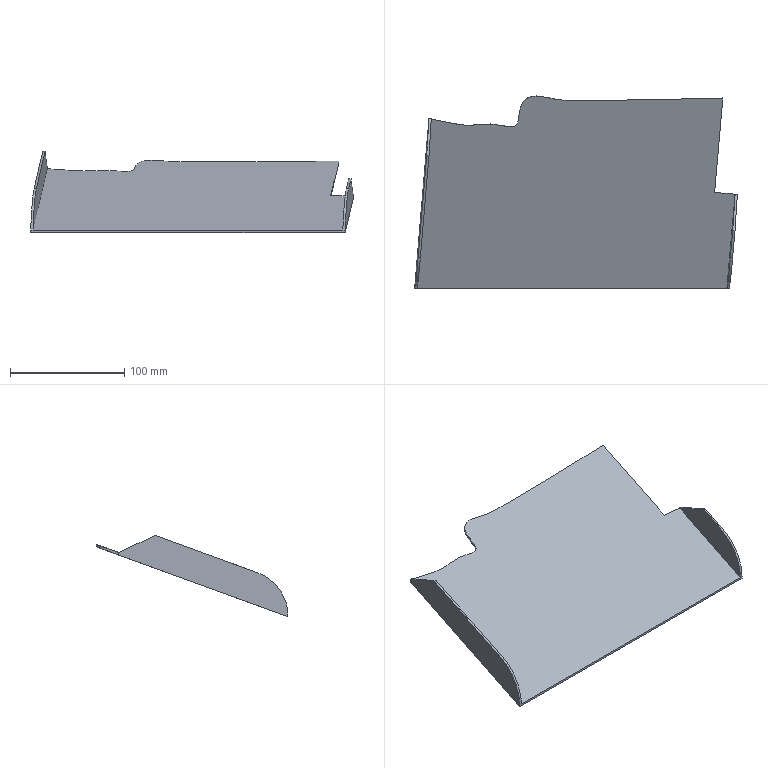Part | NX | features solid 2 | 1 solid | 18 faces | box 282.448 x 167.985 x 71.022 mm | volume 99545 mm3 | plane 15 | cylinder 2 | spline 1 | commonest cylinder face diameters 80 x2
STEP:
#1=CARTESIAN_POINT('',(-1225.198,-650.,-185.179));
#2=VERTEX_POINT('',#1);
#3=CARTESIAN_POINT('',(-953.983,-650.,-185.179));
#4=VERTEX_POINT('',#3);
#5=CARTESIAN_POINT('',(-1224.729,-650.,-185.179));
#6=DIRECTION('',(1.,0.,0.));
#7=VECTOR('',#6,1000.);
#8=LINE('',#5,#7);
#9=EDGE_CURVE('',#2,#4,#8,.T.);
#10=ORIENTED_EDGE('',*,*,#9,.T.);
#11=CARTESIAN_POINT('',(-946.807,-567.969,-155.322));
#12=VERTEX_POINT('',#11);
#13=CARTESIAN_POINT('',(-953.97,-649.846,-185.123));
#14=DIRECTION('',(0.08194,0.9365,0.3409));
#15=VECTOR('',#14,1000.);
#16=LINE('',#13,#15);
#17=EDGE_CURVE('',#4,#12,#16,.T.);
#18=ORIENTED_EDGE('',*,*,#17,.T.);
#19=CARTESIAN_POINT('',(-944.813,-568.123,-155.378));
#20=VERTEX_POINT('',#19);
#21=CARTESIAN_POINT('',(-944.813,-568.123,-155.378));
#22=DIRECTION('',(0.9966,-0.07699,-0.02802));
#23=VECTOR('',#22,1000.);
#24=LINE('',#21,#23);
#25=EDGE_CURVE('',#20,#12,#24,.F.);
#26=ORIENTED_EDGE('',*,*,#25,.F.);
#27=CARTESIAN_POINT('',(-964.737,-566.38,-154.744));
#28=VERTEX_POINT('',#27);
#29=CARTESIAN_POINT('',(-1217.161,-544.295,-146.706));
#30=DIRECTION('',(0.9957,-0.08711,-0.03171));
#31=VECTOR('',#30,1000.);
#32=LINE('',#29,#31);
#33=EDGE_CURVE('',#20,#28,#32,.F.);
#34=ORIENTED_EDGE('',*,*,#33,.T.);
#35=CARTESIAN_POINT('',(-957.511,-483.782,-124.681));
#36=VERTEX_POINT('',#35);
#37=CARTESIAN_POINT('',(-971.202,-640.27,-181.638));
#38=DIRECTION('',(-0.08194,-0.9365,-0.3409));
#39=VECTOR('',#38,1000.);
#40=LINE('',#37,#39);
#41=EDGE_CURVE('',#28,#36,#40,.F.);
#42=ORIENTED_EDGE('',*,*,#41,.T.);
#43=CARTESIAN_POINT('',(-1212.732,-502.319,-131.428));
#44=VERTEX_POINT('',#43);
#45=CARTESIAN_POINT('',(-1212.732,-502.319,-131.428));
#46=CARTESIAN_POINT('',(-1209.92,-502.972,-131.665));
#47=CARTESIAN_POINT('',(-1204.244,-504.045,-132.056));
#48=CARTESIAN_POINT('',(-1195.728,-505.629,-132.633));
#49=CARTESIAN_POINT('',(-1187.228,-507.328,-133.251));
#50=CARTESIAN_POINT('',(-1180.012,-508.008,-133.499));
#51=CARTESIAN_POINT('',(-1174.298,-507.585,-133.345));
#52=CARTESIAN_POINT('',(-1170.018,-506.973,-133.122));
#53=CARTESIAN_POINT('',(-1165.737,-506.477,-132.941));
#54=CARTESIAN_POINT('',(-1161.462,-506.397,-132.912));
#55=CARTESIAN_POINT('',(-1157.192,-506.772,-133.049));
#56=CARTESIAN_POINT('',(-1152.925,-507.483,-133.307));
#57=CARTESIAN_POINT('',(-1148.686,-508.308,-133.608));
#58=CARTESIAN_POINT('',(-1145.133,-508.877,-133.815));
#59=CARTESIAN_POINT('',(-1142.237,-508.931,-133.835));
#60=CARTESIAN_POINT('',(-1140.079,-508.546,-133.694));
#61=CARTESIAN_POINT('',(-1138.267,-507.346,-133.257));
#62=CARTESIAN_POINT('',(-1137.212,-505.531,-132.597));
#63=CARTESIAN_POINT('',(-1136.63,-503.574,-131.885));
#64=CARTESIAN_POINT('',(-1136.151,-500.931,-130.923));
#65=CARTESIAN_POINT('',(-1135.763,-497.583,-129.704));
#66=CARTESIAN_POINT('',(-1135.106,-493.616,-128.26));
#67=CARTESIAN_POINT('',(-1133.872,-489.733,-126.847));
#68=CARTESIAN_POINT('',(-1131.667,-486.211,-125.565));
#69=CARTESIAN_POINT('',(-1128.365,-483.574,-124.605));
#70=CARTESIAN_POINT('',(-1124.255,-482.166,-124.093));
#71=CARTESIAN_POINT('',(-1118.527,-481.812,-123.964));
#72=CARTESIAN_POINT('',(-1111.474,-483.246,-124.486));
#73=CARTESIAN_POINT('',(-1103.158,-485.327,-125.243));
#74=CARTESIAN_POINT('',(-1094.671,-486.054,-125.508));
#75=CARTESIAN_POINT('',(-1086.089,-485.771,-125.405));
#76=CARTESIAN_POINT('',(-1077.515,-485.65,-125.361));
#77=CARTESIAN_POINT('',(-1068.943,-485.891,-125.449));
#78=CARTESIAN_POINT('',(-1060.37,-486.017,-125.494));
#79=CARTESIAN_POINT('',(-1051.796,-485.869,-125.441));
#80=CARTESIAN_POINT('',(-1040.369,-485.599,-125.342));
#81=CARTESIAN_POINT('',(-1026.078,-485.465,-125.294));
#82=CARTESIAN_POINT('',(-1008.934,-485.128,-125.171));
#83=CARTESIAN_POINT('',(-986.076,-484.671,-125.004));
#84=CARTESIAN_POINT('',(-968.936,-484.176,-124.825));
#85=CARTESIAN_POINT('',(-957.511,-483.782,-124.681));
#86=B_SPLINE_CURVE_WITH_KNOTS('',3,(#45,#46,#47,#48,#49,#50,#51,#52,#53,#54,#55,#56,#57,#58,#59,#60,#61,#62,#63,#64,#65,#66,#67,#68,#69,#70,#71,#72,#73,#74,#75,#76,#77,#78,#79,#80,#81,#82,#83,#84,#85),.UNSPECIFIED.,.F.,.F.,(4,1,1,1,1,1,1,1,1,1,1,1,1,1,1,1,1,1,1,1,1,1,1,1,1,1,1,1,1,1,1,1,1,1,1,1,1,1,4),(0.002028,0.01071,0.01939,0.02808,0.03676,0.0411,0.04544,0.04979,0.05413,0.05847,0.06281,0.06715,0.07149,0.07367,0.07584,0.07801,0.08018,0.08235,0.08452,0.08886,0.0932,0.09754,0.1019,0.1062,0.1106,0.1149,0.1236,0.1323,0.141,0.1496,0.1583,0.167,0.1757,0.1844,0.1931,0.2104,0.2278,0.2452,0.2799),.UNSPECIFIED.);
#87=EDGE_CURVE('',#44,#36,#86,.T.);
#88=ORIENTED_EDGE('',*,*,#87,.F.);
#89=CARTESIAN_POINT('',(-1225.21,-650.149,-185.233));
#90=DIRECTION('',(0.07907,0.9368,0.3409));
#91=VECTOR('',#90,1000.);
#92=LINE('',#89,#91);
#93=EDGE_CURVE('',#2,#44,#92,.T.);
#94=ORIENTED_EDGE('',*,*,#93,.F.);
#95=EDGE_LOOP('',(#10,#18,#26,#34,#42,#88,#94));
#96=FACE_BOUND('',#95,.T.);
#97=CARTESIAN_POINT('',(-1224.729,-620.684,-174.509));
#98=DIRECTION('',(0.,0.342,-0.9397));
#99=DIRECTION('',(0.07907,0.9368,0.3409));
#100=AXIS2_PLACEMENT_3D('',#97,#98,#99);
#101=PLANE('',#100);
#102=ADVANCED_FACE('',(#96),#101,.F.);
#103=CARTESIAN_POINT('',(-1214.755,-501.827,-133.377));
#104=VERTEX_POINT('',#103);
#105=CARTESIAN_POINT('',(-957.511,-483.782,-126.809));
#106=VERTEX_POINT('',#105);
#107=CARTESIAN_POINT('',(-1214.755,-501.827,-133.377));
#108=CARTESIAN_POINT('',(-1211.964,-502.537,-133.636));
#109=CARTESIAN_POINT('',(-1206.322,-503.679,-134.051));
#110=CARTESIAN_POINT('',(-1197.817,-505.216,-134.611));
#111=CARTESIAN_POINT('',(-1189.363,-506.929,-135.234));
#112=CARTESIAN_POINT('',(-1182.184,-507.906,-135.59));
#113=CARTESIAN_POINT('',(-1176.473,-507.801,-135.552));
#114=CARTESIAN_POINT('',(-1172.204,-507.299,-135.369));
#115=CARTESIAN_POINT('',(-1167.936,-506.692,-135.148));
#116=CARTESIAN_POINT('',(-1163.67,-506.379,-135.034));
#117=CARTESIAN_POINT('',(-1159.41,-506.525,-135.087));
#118=CARTESIAN_POINT('',(-1155.148,-507.083,-135.29));
#119=CARTESIAN_POINT('',(-1150.91,-507.875,-135.578));
#120=CARTESIAN_POINT('',(-1147.381,-508.541,-135.821));
#121=CARTESIAN_POINT('',(-1144.534,-508.882,-135.945));
#122=CARTESIAN_POINT('',(-1142.368,-508.937,-135.965));
#123=CARTESIAN_POINT('',(-1140.209,-508.589,-135.839));
#124=CARTESIAN_POINT('',(-1138.36,-507.446,-135.422));
#125=CARTESIAN_POINT('',(-1137.262,-505.658,-134.772));
#126=CARTESIAN_POINT('',(-1136.463,-503.057,-133.825));
#127=CARTESIAN_POINT('',(-1136.016,-499.737,-132.616));
#128=CARTESIAN_POINT('',(-1135.502,-495.735,-131.16));
#129=CARTESIAN_POINT('',(-1134.638,-491.824,-129.736));
#130=CARTESIAN_POINT('',(-1133.006,-488.055,-128.364));
#131=CARTESIAN_POINT('',(-1130.284,-484.863,-127.203));
#132=CARTESIAN_POINT('',(-1126.547,-482.769,-126.441));
#133=CARTESIAN_POINT('',(-1120.866,-481.647,-126.032));
#134=CARTESIAN_POINT('',(-1113.743,-482.64,-126.394));
#135=CARTESIAN_POINT('',(-1105.393,-484.866,-127.204));
#136=CARTESIAN_POINT('',(-1096.872,-486.017,-127.623));
#137=CARTESIAN_POINT('',(-1088.16,-485.861,-127.566));
#138=CARTESIAN_POINT('',(-1079.444,-485.631,-127.482));
#139=CARTESIAN_POINT('',(-1070.731,-485.835,-127.556));
#140=CARTESIAN_POINT('',(-1059.112,-486.08,-127.646));
#141=CARTESIAN_POINT('',(-1044.598,-485.649,-127.489));
#142=CARTESIAN_POINT('',(-1027.176,-485.478,-127.427));
#143=CARTESIAN_POINT('',(-1009.757,-485.147,-127.306));
#144=CARTESIAN_POINT('',(-986.533,-484.68,-127.136));
#145=CARTESIAN_POINT('',(-969.118,-484.183,-126.955));
#146=CARTESIAN_POINT('',(-957.511,-483.782,-126.809));
#147=B_SPLINE_CURVE_WITH_KNOTS('',3,(#107,#108,#109,#110,#111,#112,#113,#114,#115,#116,#117,#118,#119,#120,#121,#122,#123,#124,#125,#126,#127,#128,#129,#130,#131,#132,#133,#134,#135,#136,#137,#138,#139,#140,#141,#142,#143,#144,#145,#146),.UNSPECIFIED.,.F.,.F.,(4,1,1,1,1,1,1,1,1,1,1,1,1,1,1,1,1,1,1,1,1,1,1,1,1,1,1,1,1,1,1,1,1,1,1,1,1,4),(0.,0.008657,0.01731,0.02597,0.03463,0.03896,0.04329,0.04761,0.05194,0.05627,0.0606,0.06493,0.06926,0.07142,0.07359,0.07575,0.07791,0.08008,0.08224,0.08657,0.0909,0.09523,0.09956,0.1039,0.1082,0.1125,0.1212,0.1299,0.1385,0.1472,0.1558,0.1645,0.1731,0.1905,0.2078,0.2251,0.2424,0.277),.UNSPECIFIED.);
#148=EDGE_CURVE('',#104,#106,#147,.T.);
#149=ORIENTED_EDGE('',*,*,#148,.T.);
#150=CARTESIAN_POINT('',(-964.737,-566.38,-156.872));
#151=VERTEX_POINT('',#150);
#152=CARTESIAN_POINT('',(-971.142,-639.591,-183.519));
#153=DIRECTION('',(-0.08194,-0.9365,-0.3409));
#154=VECTOR('',#153,1000.);
#155=LINE('',#152,#154);
#156=EDGE_CURVE('',#106,#151,#155,.T.);
#157=ORIENTED_EDGE('',*,*,#156,.T.);
#158=CARTESIAN_POINT('',(-944.813,-568.123,-157.507));
#159=VERTEX_POINT('',#158);
#160=CARTESIAN_POINT('',(33.81,-653.741,-188.669));
#161=DIRECTION('',(-0.9957,0.08711,0.03171));
#162=VECTOR('',#161,1000.);
#163=LINE('',#160,#162);
#164=EDGE_CURVE('',#151,#159,#163,.F.);
#165=ORIENTED_EDGE('',*,*,#164,.T.);
#166=CARTESIAN_POINT('',(-951.977,-650.,-187.308));
#167=VERTEX_POINT('',#166);
#168=CARTESIAN_POINT('',(-936.476,-472.827,-122.822));
#169=DIRECTION('',(0.08194,0.9365,0.3409));
#170=VECTOR('',#169,1000.);
#171=LINE('',#168,#170);
#172=EDGE_CURVE('',#167,#159,#171,.T.);
#173=ORIENTED_EDGE('',*,*,#172,.F.);
#174=CARTESIAN_POINT('',(-1227.262,-650.,-187.308));
#175=VERTEX_POINT('',#174);
#176=CARTESIAN_POINT('',(50.,-650.,-187.308));
#177=DIRECTION('',(-1.,0.,0.));
#178=VECTOR('',#177,1000.);
#179=LINE('',#176,#178);
#180=EDGE_CURVE('',#175,#167,#179,.F.);
#181=ORIENTED_EDGE('',*,*,#180,.F.);
#182=CARTESIAN_POINT('',(-1224.729,-620.,-176.389));
#183=DIRECTION('',(0.07907,0.9368,0.3409));
#184=VECTOR('',#183,1000.);
#185=LINE('',#182,#184);
#186=EDGE_CURVE('',#175,#104,#185,.T.);
#187=ORIENTED_EDGE('',*,*,#186,.T.);
#188=EDGE_LOOP('',(#149,#157,#165,#173,#181,#187));
#189=FACE_BOUND('',#188,.T.);
#190=CARTESIAN_POINT('',(-1224.729,-620.,-176.389));
#191=DIRECTION('',(0.,0.342,-0.9397));
#192=DIRECTION('',(0.07907,0.9368,0.3409));
#193=AXIS2_PLACEMENT_3D('',#190,#191,#192);
#194=PLANE('',#193);
#195=ADVANCED_FACE('',(#189),#194,.T.);
#196=CARTESIAN_POINT('',(-1214.698,-501.841,-131.254));
#197=VERTEX_POINT('',#196);
#198=CARTESIAN_POINT('',(-1214.698,-501.841,-131.254));
#199=CARTESIAN_POINT('',(-1214.044,-502.007,-131.315));
#200=CARTESIAN_POINT('',(-1213.389,-502.166,-131.372));
#201=CARTESIAN_POINT('',(-1212.732,-502.319,-131.428));
#202=B_SPLINE_CURVE_WITH_KNOTS('',3,(#198,#199,#200,#201),.UNSPECIFIED.,.F.,.F.,(4,4),(0.,0.002028),.UNSPECIFIED.);
#203=EDGE_CURVE('',#197,#44,#202,.T.);
#204=ORIENTED_EDGE('',*,*,#203,.T.);
#205=ORIENTED_EDGE('',*,*,#87,.T.);
#206=CARTESIAN_POINT('',(-957.511,-483.782,-129.983));
#207=DIRECTION('',(0.,0.,1.));
#208=VECTOR('',#207,1000.);
#209=LINE('',#206,#208);
#210=EDGE_CURVE('',#36,#106,#209,.F.);
#211=ORIENTED_EDGE('',*,*,#210,.T.);
#212=ORIENTED_EDGE('',*,*,#148,.F.);
#213=CARTESIAN_POINT('',(-1214.755,-501.827,-133.377));
#214=CARTESIAN_POINT('',(-1214.736,-501.832,-132.67));
#215=CARTESIAN_POINT('',(-1214.717,-501.837,-131.962));
#216=CARTESIAN_POINT('',(-1214.698,-501.841,-131.254));
#217=B_SPLINE_CURVE_WITH_KNOTS('',3,(#213,#214,#215,#216),.UNSPECIFIED.,.F.,.F.,(4,4),(0.,0.002124),.UNSPECIFIED.);
#218=EDGE_CURVE('',#104,#197,#217,.T.);
#219=ORIENTED_EDGE('',*,*,#218,.T.);
#220=EDGE_LOOP('',(#204,#205,#211,#212,#219));
#221=FACE_BOUND('',#220,.T.);
#222=CARTESIAN_POINT('',(-1216.33,-501.411,-136.024));
#223=CARTESIAN_POINT('',(-1216.33,-501.411,-123.942));
#224=CARTESIAN_POINT('',(-1213.583,-502.164,-136.024));
#225=CARTESIAN_POINT('',(-1213.583,-502.164,-123.942));
#226=CARTESIAN_POINT('',(-1208.051,-503.37,-136.024));
#227=CARTESIAN_POINT('',(-1208.051,-503.37,-123.942));
#228=CARTESIAN_POINT('',(-1199.467,-504.899,-136.024));
#229=CARTESIAN_POINT('',(-1199.467,-504.899,-123.942));
#230=CARTESIAN_POINT('',(-1190.511,-506.704,-136.024));
#231=CARTESIAN_POINT('',(-1190.511,-506.704,-123.942));
#232=CARTESIAN_POINT('',(-1181.633,-508.067,-136.024));
#233=CARTESIAN_POINT('',(-1181.633,-508.067,-123.942));
#234=CARTESIAN_POINT('',(-1173.473,-507.596,-136.024));
#235=CARTESIAN_POINT('',(-1173.473,-507.596,-123.942));
#236=CARTESIAN_POINT('',(-1166.687,-506.432,-136.024));
#237=CARTESIAN_POINT('',(-1166.687,-506.432,-123.942));
#238=CARTESIAN_POINT('',(-1160.524,-506.423,-136.024));
#239=CARTESIAN_POINT('',(-1160.524,-506.423,-123.942));
#240=CARTESIAN_POINT('',(-1153.877,-507.185,-136.024));
#241=CARTESIAN_POINT('',(-1153.877,-507.185,-123.942));
#242=CARTESIAN_POINT('',(-1146.929,-508.795,-136.024));
#243=CARTESIAN_POINT('',(-1146.929,-508.795,-123.942));
#244=CARTESIAN_POINT('',(-1141.555,-509.015,-136.024));
#245=CARTESIAN_POINT('',(-1141.555,-509.015,-123.942));
#246=CARTESIAN_POINT('',(-1138.685,-507.939,-136.024));
#247=CARTESIAN_POINT('',(-1138.685,-507.939,-123.942));
#248=CARTESIAN_POINT('',(-1137.024,-505.415,-136.024));
#249=CARTESIAN_POINT('',(-1137.024,-505.415,-123.942));
#250=CARTESIAN_POINT('',(-1135.968,-500.412,-136.024));
#251=CARTESIAN_POINT('',(-1135.968,-500.412,-123.942));
#252=CARTESIAN_POINT('',(-1135.329,-492.338,-136.024));
#253=CARTESIAN_POINT('',(-1135.329,-492.338,-123.942));
#254=CARTESIAN_POINT('',(-1131.162,-484.704,-136.024));
#255=CARTESIAN_POINT('',(-1131.162,-484.704,-123.942));
#256=CARTESIAN_POINT('',(-1123.528,-481.546,-136.024));
#257=CARTESIAN_POINT('',(-1123.528,-481.546,-123.942));
#258=CARTESIAN_POINT('',(-1114.821,-482.354,-136.024));
#259=CARTESIAN_POINT('',(-1114.821,-482.354,-123.942));
#260=CARTESIAN_POINT('',(-1106.183,-484.691,-136.024));
#261=CARTESIAN_POINT('',(-1106.183,-484.691,-123.942));
#262=CARTESIAN_POINT('',(-1097.521,-485.994,-136.024));
#263=CARTESIAN_POINT('',(-1097.521,-485.994,-123.942));
#264=CARTESIAN_POINT('',(-1088.741,-485.887,-136.024));
#265=CARTESIAN_POINT('',(-1088.741,-485.887,-123.942));
#266=CARTESIAN_POINT('',(-1079.955,-485.63,-136.024));
#267=CARTESIAN_POINT('',(-1079.955,-485.63,-123.942));
#268=CARTESIAN_POINT('',(-1071.218,-485.818,-136.024));
#269=CARTESIAN_POINT('',(-1071.218,-485.818,-123.942));
#270=CARTESIAN_POINT('',(-1059.579,-486.085,-136.024));
#271=CARTESIAN_POINT('',(-1059.579,-486.085,-123.942));
#272=CARTESIAN_POINT('',(-1044.974,-485.659,-136.024));
#273=CARTESIAN_POINT('',(-1044.974,-485.659,-123.942));
#274=CARTESIAN_POINT('',(-1027.488,-485.48,-136.024));
#275=CARTESIAN_POINT('',(-1027.488,-485.48,-123.942));
#276=CARTESIAN_POINT('',(-1009.988,-485.152,-136.024));
#277=CARTESIAN_POINT('',(-1009.988,-485.152,-123.942));
#278=CARTESIAN_POINT('',(-986.661,-484.683,-136.024));
#279=CARTESIAN_POINT('',(-986.661,-484.683,-123.942));
#280=CARTESIAN_POINT('',(-969.169,-484.184,-136.024));
#281=CARTESIAN_POINT('',(-969.169,-484.184,-123.942));
#282=CARTESIAN_POINT('',(-957.511,-483.782,-136.024));
#283=CARTESIAN_POINT('',(-957.511,-483.782,-123.942));
#284=B_SPLINE_SURFACE_WITH_KNOTS('',3,1,((#222,#223),(#224,#225),(#226,#227),(#228,#229),(#230,#231),(#232,#233),(#234,#235),(#236,#237),(#238,#239),(#240,#241),(#242,#243),(#244,#245),(#246,#247),(#248,#249),(#250,#251),(#252,#253),(#254,#255),(#256,#257),(#258,#259),(#260,#261),(#262,#263),(#264,#265),(#266,#267),(#268,#269),(#270,#271),(#272,#273),(#274,#275),(#276,#277),(#278,#279),(#280,#281),(#282,#283)),.SURF_OF_LINEAR_EXTRUSION.,.F.,.F.,.F.,(4,1,1,1,1,1,1,1,1,1,1,1,1,1,1,1,1,1,1,1,1,1,1,1,1,1,1,1,4),(2,2),(0.004003,0.006289,0.008575,0.01086,0.01315,0.01543,0.01772,0.01886,0.02001,0.02229,0.02343,0.02458,0.02572,0.02686,0.02915,0.03144,0.03372,0.03601,0.03829,0.04058,0.04287,0.04515,0.04744,0.04973,0.0543,0.05887,0.06344,0.06801,0.07716),(0.,1.),.UNSPECIFIED.);
#285=ADVANCED_FACE('',(#221),#284,.F.);
#286=ORIENTED_EDGE('',*,*,#172,.T.);
#287=CARTESIAN_POINT('',(-944.813,-568.123,-110.));
#288=DIRECTION('',(0.,0.,1.));
#289=VECTOR('',#288,1000.);
#290=LINE('',#287,#289);
#291=EDGE_CURVE('',#159,#20,#290,.T.);
#292=ORIENTED_EDGE('',*,*,#291,.T.);
#293=CARTESIAN_POINT('',(-951.977,-650.,-185.179));
#294=VERTEX_POINT('',#293);
#295=CARTESIAN_POINT('',(-951.26,-641.811,-182.199));
#296=DIRECTION('',(-0.08194,-0.9365,-0.3409));
#297=VECTOR('',#296,1000.);
#298=LINE('',#295,#297);
#299=EDGE_CURVE('',#294,#20,#298,.F.);
#300=ORIENTED_EDGE('',*,*,#299,.F.);
#301=CARTESIAN_POINT('',(-951.977,-650.,-570.));
#302=DIRECTION('',(0.,0.,-1.));
#303=VECTOR('',#302,1000.);
#304=LINE('',#301,#303);
#305=EDGE_CURVE('',#167,#294,#304,.F.);
#306=ORIENTED_EDGE('',*,*,#305,.F.);
#307=EDGE_LOOP('',(#286,#292,#300,#306));
#308=FACE_BOUND('',#307,.T.);
#309=CARTESIAN_POINT('',(-936.881,-477.458,-110.));
#310=DIRECTION('',(0.9962,-0.08716,0.));
#311=DIRECTION('',(0.08716,0.9962,0.));
#312=AXIS2_PLACEMENT_3D('',#309,#310,#311);
#313=PLANE('',#312);
#314=ADVANCED_FACE('',(#308),#313,.T.);
#315=CARTESIAN_POINT('',(-1227.204,-650.,-185.179));
#316=VERTEX_POINT('',#315);
#317=CARTESIAN_POINT('',(-1236.696,-650.,-535.095));
#318=DIRECTION('',(-0.02712,0.,-0.9996));
#319=VECTOR('',#318,1000.);
#320=LINE('',#317,#319);
#321=EDGE_CURVE('',#175,#316,#320,.F.);
#322=ORIENTED_EDGE('',*,*,#321,.F.);
#323=ORIENTED_EDGE('',*,*,#180,.T.);
#324=ORIENTED_EDGE('',*,*,#305,.T.);
#325=CARTESIAN_POINT('',(-951.977,-650.,-185.179));
#326=DIRECTION('',(1.,0.,0.));
#327=VECTOR('',#326,1000.);
#328=LINE('',#325,#327);
#329=EDGE_CURVE('',#294,#4,#328,.F.);
#330=ORIENTED_EDGE('',*,*,#329,.T.);
#331=ORIENTED_EDGE('',*,*,#9,.F.);
#332=CARTESIAN_POINT('',(-1224.729,-650.,-185.179));
#333=DIRECTION('',(1.,0.,0.));
#334=VECTOR('',#333,1000.);
#335=LINE('',#332,#334);
#336=EDGE_CURVE('',#316,#2,#335,.T.);
#337=ORIENTED_EDGE('',*,*,#336,.F.);
#338=EDGE_LOOP('',(#322,#323,#324,#330,#331,#337));
#339=FACE_BOUND('',#338,.T.);
#340=CARTESIAN_POINT('',(50.,-650.,-570.));
#341=DIRECTION('',(0.,1.,0.));
#342=DIRECTION('',(-1.,0.,0.));
#343=AXIS2_PLACEMENT_3D('',#340,#341,#342);
#344=PLANE('',#343);
#345=ADVANCED_FACE('',(#339),#344,.F.);
#346=ORIENTED_EDGE('',*,*,#321,.T.);
#347=CARTESIAN_POINT('',(-1224.263,-623.706,-149.005));
#348=VERTEX_POINT('',#347);
#349=CARTESIAN_POINT('',(-1224.263,-610.025,-186.592));
#350=DIRECTION('',(0.9969,-0.0743,-0.02704));
#351=DIRECTION('',(-0.07907,-0.9368,-0.3409));
#352=AXIS2_PLACEMENT_3D('',#349,#350,#351);
#353=ELLIPSE('',#352,40.126,40.);
#354=EDGE_CURVE('',#316,#348,#353,.F.);
#355=ORIENTED_EDGE('',*,*,#354,.T.);
#356=CARTESIAN_POINT('',(-1216.675,-533.811,-116.286));
#357=VERTEX_POINT('',#356);
#358=CARTESIAN_POINT('',(-1227.204,-658.551,-161.687));
#359=DIRECTION('',(0.07907,0.9368,0.3409));
#360=VECTOR('',#359,1000.);
#361=LINE('',#358,#360);
#362=EDGE_CURVE('',#348,#357,#361,.T.);
#363=ORIENTED_EDGE('',*,*,#362,.T.);
#364=CARTESIAN_POINT('',(-1214.698,-501.841,-131.254));
#365=DIRECTION('',(0.05591,0.9042,-0.4234));
#366=VECTOR('',#365,1000.);
#367=LINE('',#364,#366);
#368=EDGE_CURVE('',#357,#197,#367,.T.);
#369=ORIENTED_EDGE('',*,*,#368,.T.);
#370=ORIENTED_EDGE('',*,*,#218,.F.);
#371=ORIENTED_EDGE('',*,*,#186,.F.);
#372=EDGE_LOOP('',(#346,#355,#363,#369,#370,#371));
#373=FACE_BOUND('',#372,.T.);
#374=CARTESIAN_POINT('',(-1224.729,-620.,-176.389));
#375=DIRECTION('',(0.9969,-0.0743,-0.02704));
#376=DIRECTION('',(0.07433,0.9972,0.));
#377=AXIS2_PLACEMENT_3D('',#374,#375,#376);
#378=PLANE('',#377);
#379=ADVANCED_FACE('',(#373),#378,.F.);
#380=ORIENTED_EDGE('',*,*,#210,.F.);
#381=ORIENTED_EDGE('',*,*,#41,.F.);
#382=CARTESIAN_POINT('',(-964.737,-566.38,-38.668));
#383=DIRECTION('',(0.,0.,1.));
#384=VECTOR('',#383,1000.);
#385=LINE('',#382,#384);
#386=EDGE_CURVE('',#151,#28,#385,.T.);
#387=ORIENTED_EDGE('',*,*,#386,.F.);
#388=ORIENTED_EDGE('',*,*,#156,.F.);
#389=EDGE_LOOP('',(#380,#381,#387,#388));
#390=FACE_BOUND('',#389,.T.);
#391=CARTESIAN_POINT('',(-947.306,-367.141,-38.668));
#392=DIRECTION('',(0.9962,-0.08716,0.));
#393=DIRECTION('',(0.08716,0.9962,0.));
#394=AXIS2_PLACEMENT_3D('',#391,#392,#393);
#395=PLANE('',#394);
#396=ADVANCED_FACE('',(#390),#395,.T.);
#397=ORIENTED_EDGE('',*,*,#291,.F.);
#398=ORIENTED_EDGE('',*,*,#164,.F.);
#399=ORIENTED_EDGE('',*,*,#386,.T.);
#400=ORIENTED_EDGE('',*,*,#33,.F.);
#401=EDGE_LOOP('',(#397,#398,#399,#400));
#402=FACE_BOUND('',#401,.T.);
#403=CARTESIAN_POINT('',(-964.737,-566.38,-38.668));
#404=DIRECTION('',(0.08716,0.9962,0.));
#405=DIRECTION('',(-0.9962,0.08716,0.));
#406=AXIS2_PLACEMENT_3D('',#403,#404,#405);
#407=PLANE('',#406);
#408=ADVANCED_FACE('',(#402),#407,.T.);
#409=CARTESIAN_POINT('',(-1212.705,-501.99,-131.308));
#410=VERTEX_POINT('',#409);
#411=CARTESIAN_POINT('',(-1225.21,-650.149,-185.233));
#412=DIRECTION('',(0.07907,0.9368,0.3409));
#413=VECTOR('',#412,1000.);
#414=LINE('',#411,#413);
#415=EDGE_CURVE('',#44,#410,#414,.T.);
#416=ORIENTED_EDGE('',*,*,#415,.F.);
#417=ORIENTED_EDGE('',*,*,#203,.F.);
#418=CARTESIAN_POINT('',(-1214.698,-501.841,-131.254));
#419=DIRECTION('',(0.9969,-0.0743,-0.02704));
#420=VECTOR('',#419,1000.);
#421=LINE('',#418,#420);
#422=EDGE_CURVE('',#197,#410,#421,.T.);
#423=ORIENTED_EDGE('',*,*,#422,.T.);
#424=EDGE_LOOP('',(#416,#417,#423));
#425=FACE_BOUND('',#424,.T.);
#426=CARTESIAN_POINT('',(-1227.204,-650.,-185.179));
#427=DIRECTION('',(0.,0.342,-0.9397));
#428=DIRECTION('',(0.07907,0.9368,0.3409));
#429=AXIS2_PLACEMENT_3D('',#426,#427,#428);
#430=PLANE('',#429);
#431=ADVANCED_FACE('',(#425),#430,.T.);
#432=CARTESIAN_POINT('',(-1222.257,-623.706,-149.005));
#433=VERTEX_POINT('',#432);
#434=CARTESIAN_POINT('',(-1214.681,-533.959,-116.34));
#435=VERTEX_POINT('',#434);
#436=CARTESIAN_POINT('',(-1225.21,-658.699,-161.741));
#437=DIRECTION('',(0.07907,0.9368,0.3409));
#438=VECTOR('',#437,1000.);
#439=LINE('',#436,#438);
#440=EDGE_CURVE('',#433,#435,#439,.T.);
#441=ORIENTED_EDGE('',*,*,#440,.T.);
#442=CARTESIAN_POINT('',(-1216.675,-533.811,-116.286));
#443=DIRECTION('',(0.9969,-0.0743,-0.02704));
#444=VECTOR('',#443,1000.);
#445=LINE('',#442,#444);
#446=EDGE_CURVE('',#435,#357,#445,.F.);
#447=ORIENTED_EDGE('',*,*,#446,.T.);
#448=ORIENTED_EDGE('',*,*,#362,.F.);
#449=CARTESIAN_POINT('',(-1224.476,-623.706,-149.005));
#450=DIRECTION('',(-1.,0.,0.));
#451=VECTOR('',#450,1000.);
#452=LINE('',#449,#451);
#453=EDGE_CURVE('',#348,#433,#452,.F.);
#454=ORIENTED_EDGE('',*,*,#453,.T.);
#455=EDGE_LOOP('',(#441,#447,#448,#454));
#456=FACE_BOUND('',#455,.T.);
#457=CARTESIAN_POINT('',(-1227.204,-658.551,-161.687));
#458=DIRECTION('',(0.,0.342,-0.9397));
#459=DIRECTION('',(0.07907,0.9368,0.3409));
#460=AXIS2_PLACEMENT_3D('',#457,#458,#459);
#461=PLANE('',#460);
#462=ADVANCED_FACE('',(#456),#461,.F.);
#463=ORIENTED_EDGE('',*,*,#93,.T.);
#464=ORIENTED_EDGE('',*,*,#415,.T.);
#465=CARTESIAN_POINT('',(-1218.957,-603.117,-83.959));
#466=DIRECTION('',(-0.05591,-0.9042,0.4234));
#467=VECTOR('',#466,1000.);
#468=LINE('',#465,#467);
#469=EDGE_CURVE('',#410,#435,#468,.T.);
#470=ORIENTED_EDGE('',*,*,#469,.T.);
#471=ORIENTED_EDGE('',*,*,#440,.F.);
#472=CARTESIAN_POINT('',(-1222.257,-610.025,-186.592));
#473=DIRECTION('',(0.9969,-0.0743,-0.02704));
#474=DIRECTION('',(-0.07907,-0.9368,-0.3409));
#475=AXIS2_PLACEMENT_3D('',#472,#473,#474);
#476=ELLIPSE('',#475,40.126,40.);
#477=EDGE_CURVE('',#433,#2,#476,.T.);
#478=ORIENTED_EDGE('',*,*,#477,.T.);
#479=EDGE_LOOP('',(#463,#464,#470,#471,#478));
#480=FACE_BOUND('',#479,.T.);
#481=CARTESIAN_POINT('',(-1225.21,-650.149,-185.233));
#482=DIRECTION('',(0.9969,-0.0743,-0.02704));
#483=DIRECTION('',(0.07433,0.9972,0.));
#484=AXIS2_PLACEMENT_3D('',#481,#482,#483);
#485=PLANE('',#484);
#486=ADVANCED_FACE('',(#480),#485,.T.);
#487=ORIENTED_EDGE('',*,*,#354,.F.);
#488=ORIENTED_EDGE('',*,*,#336,.T.);
#489=ORIENTED_EDGE('',*,*,#477,.F.);
#490=ORIENTED_EDGE('',*,*,#453,.F.);
#491=EDGE_LOOP('',(#487,#488,#489,#490));
#492=FACE_BOUND('',#491,.T.);
#493=CARTESIAN_POINT('',(50.,-610.025,-186.592));
#494=DIRECTION('',(-1.,0.,0.));
#495=DIRECTION('',(0.,0.,1.));
#496=AXIS2_PLACEMENT_3D('',#493,#494,#495);
#497=CYLINDRICAL_SURFACE('',#496,40.);
#498=ADVANCED_FACE('',(#492),#497,.T.);
#499=ORIENTED_EDGE('',*,*,#368,.F.);
#500=ORIENTED_EDGE('',*,*,#446,.F.);
#501=ORIENTED_EDGE('',*,*,#469,.F.);
#502=ORIENTED_EDGE('',*,*,#422,.F.);
#503=EDGE_LOOP('',(#499,#500,#501,#502));
#504=FACE_BOUND('',#503,.T.);
#505=CARTESIAN_POINT('',(-1214.698,-501.841,-131.254));
#506=DIRECTION('',(0.05591,0.4205,0.9056));
#507=DIRECTION('',(0.,-0.907,0.4212));
#508=AXIS2_PLACEMENT_3D('',#505,#506,#507);
#509=PLANE('',#508);
#510=ADVANCED_FACE('',(#504),#509,.T.);
#511=CARTESIAN_POINT('',(-948.928,-623.706,-149.005));
#512=VERTEX_POINT('',#511);
#513=CARTESIAN_POINT('',(-946.862,-600.087,-140.408));
#514=VERTEX_POINT('',#513);
#515=CARTESIAN_POINT('',(-951.977,-658.551,-161.687));
#516=DIRECTION('',(0.08194,0.9365,0.3409));
#517=VECTOR('',#516,1000.);
#518=LINE('',#515,#517);
#519=EDGE_CURVE('',#512,#514,#518,.T.);
#520=ORIENTED_EDGE('',*,*,#519,.T.);
#521=CARTESIAN_POINT('',(-948.855,-599.933,-140.352));
#522=VERTEX_POINT('',#521);
#523=CARTESIAN_POINT('',(-946.862,-600.087,-140.408));
#524=DIRECTION('',(-0.9966,0.07699,0.02802));
#525=VECTOR('',#524,1000.);
#526=LINE('',#523,#525);
#527=EDGE_CURVE('',#514,#522,#526,.T.);
#528=ORIENTED_EDGE('',*,*,#527,.T.);
#529=CARTESIAN_POINT('',(-950.935,-623.706,-149.005));
#530=VERTEX_POINT('',#529);
#531=CARTESIAN_POINT('',(-953.97,-658.397,-161.631));
#532=DIRECTION('',(0.08194,0.9365,0.3409));
#533=VECTOR('',#532,1000.);
#534=LINE('',#531,#533);
#535=EDGE_CURVE('',#530,#522,#534,.T.);
#536=ORIENTED_EDGE('',*,*,#535,.F.);
#537=CARTESIAN_POINT('',(-951.977,-623.706,-149.005));
#538=DIRECTION('',(-1.,0.,0.));
#539=VECTOR('',#538,1000.);
#540=LINE('',#537,#539);
#541=EDGE_CURVE('',#530,#512,#540,.F.);
#542=ORIENTED_EDGE('',*,*,#541,.T.);
#543=EDGE_LOOP('',(#520,#528,#536,#542));
#544=FACE_BOUND('',#543,.T.);
#545=CARTESIAN_POINT('',(-951.977,-658.551,-161.687));
#546=DIRECTION('',(0.,0.342,-0.9397));
#547=DIRECTION('',(0.08194,0.9365,0.3409));
#548=AXIS2_PLACEMENT_3D('',#545,#546,#547);
#549=PLANE('',#548);
#550=ADVANCED_FACE('',(#544),#549,.F.);
#551=ORIENTED_EDGE('',*,*,#535,.T.);
#552=CARTESIAN_POINT('',(-948.855,-599.933,-140.352));
#553=DIRECTION('',(0.05794,0.9041,-0.4234));
#554=VECTOR('',#553,1000.);
#555=LINE('',#552,#554);
#556=EDGE_CURVE('',#522,#12,#555,.T.);
#557=ORIENTED_EDGE('',*,*,#556,.T.);
#558=ORIENTED_EDGE('',*,*,#17,.F.);
#559=CARTESIAN_POINT('',(-950.935,-610.025,-186.592));
#560=DIRECTION('',(0.9966,-0.07699,-0.02802));
#561=DIRECTION('',(-0.08194,-0.9365,-0.3409));
#562=AXIS2_PLACEMENT_3D('',#559,#560,#561);
#563=ELLIPSE('',#562,40.135,40.);
#564=EDGE_CURVE('',#4,#530,#563,.F.);
#565=ORIENTED_EDGE('',*,*,#564,.T.);
#566=EDGE_LOOP('',(#551,#557,#558,#565));
#567=FACE_BOUND('',#566,.T.);
#568=CARTESIAN_POINT('',(-953.97,-649.846,-185.123));
#569=DIRECTION('',(0.9966,-0.07699,-0.02802));
#570=DIRECTION('',(0.07702,0.997,0.));
#571=AXIS2_PLACEMENT_3D('',#568,#569,#570);
#572=PLANE('',#571);
#573=ADVANCED_FACE('',(#567),#572,.F.);
#574=ORIENTED_EDGE('',*,*,#299,.T.);
#575=CARTESIAN_POINT('',(-948.395,-624.012,-129.202));
#576=DIRECTION('',(-0.05794,-0.9041,0.4234));
#577=VECTOR('',#576,1000.);
#578=LINE('',#575,#577);
#579=EDGE_CURVE('',#20,#514,#578,.T.);
#580=ORIENTED_EDGE('',*,*,#579,.T.);
#581=ORIENTED_EDGE('',*,*,#519,.F.);
#582=CARTESIAN_POINT('',(-948.928,-610.025,-186.592));
#583=DIRECTION('',(0.9966,-0.07699,-0.02802));
#584=DIRECTION('',(-0.08194,-0.9365,-0.3409));
#585=AXIS2_PLACEMENT_3D('',#582,#583,#584);
#586=ELLIPSE('',#585,40.135,40.);
#587=EDGE_CURVE('',#512,#294,#586,.T.);
#588=ORIENTED_EDGE('',*,*,#587,.T.);
#589=EDGE_LOOP('',(#574,#580,#581,#588));
#590=FACE_BOUND('',#589,.T.);
#591=CARTESIAN_POINT('',(-951.977,-650.,-185.179));
#592=DIRECTION('',(0.9966,-0.07699,-0.02802));
#593=DIRECTION('',(0.07702,0.997,0.));
#594=AXIS2_PLACEMENT_3D('',#591,#592,#593);
#595=PLANE('',#594);
#596=ADVANCED_FACE('',(#590),#595,.T.);
#597=ORIENTED_EDGE('',*,*,#587,.F.);
#598=ORIENTED_EDGE('',*,*,#541,.F.);
#599=ORIENTED_EDGE('',*,*,#564,.F.);
#600=ORIENTED_EDGE('',*,*,#329,.F.);
#601=EDGE_LOOP('',(#597,#598,#599,#600));
#602=FACE_BOUND('',#601,.T.);
#603=CARTESIAN_POINT('',(50.,-610.025,-186.592));
#604=DIRECTION('',(-1.,0.,0.));
#605=DIRECTION('',(0.,0.,1.));
#606=AXIS2_PLACEMENT_3D('',#603,#604,#605);
#607=CYLINDRICAL_SURFACE('',#606,40.);
#608=ADVANCED_FACE('',(#602),#607,.T.);
#609=ORIENTED_EDGE('',*,*,#579,.F.);
#610=ORIENTED_EDGE('',*,*,#25,.T.);
#611=ORIENTED_EDGE('',*,*,#556,.F.);
#612=ORIENTED_EDGE('',*,*,#527,.F.);
#613=EDGE_LOOP('',(#609,#610,#611,#612));
#614=FACE_BOUND('',#613,.T.);
#615=CARTESIAN_POINT('',(-946.862,-600.087,-140.408));
#616=DIRECTION('',(0.05794,0.4204,0.9055));
#617=DIRECTION('',(0.,-0.907,0.4211));
#618=AXIS2_PLACEMENT_3D('',#615,#616,#617);
#619=PLANE('',#618);
#620=ADVANCED_FACE('',(#614),#619,.T.);
#621=CLOSED_SHELL('',(#102,#195,#285,#314,#345,#379,#396,#408,#431,#462,#486,#498,#510,#550,#573,#596,#608,#620));
#622=MANIFOLD_SOLID_BREP('',#621);
#623=(LENGTH_UNIT()NAMED_UNIT(*)SI_UNIT(.MILLI.,.METRE.));
#624=UNCERTAINTY_MEASURE_WITH_UNIT(LENGTH_MEASURE(0.0508),#623,'','');
#625=(NAMED_UNIT(*)PLANE_ANGLE_UNIT()SI_UNIT($,.RADIAN.));
#626=(NAMED_UNIT(*)SI_UNIT($,.STERADIAN.)SOLID_ANGLE_UNIT());
#627=(GEOMETRIC_REPRESENTATION_CONTEXT(3)GLOBAL_UNCERTAINTY_ASSIGNED_CONTEXT((#624))GLOBAL_UNIT_ASSIGNED_CONTEXT((#623,#625,#626))REPRESENTATION_CONTEXT('',''));
#628=ADVANCED_BREP_SHAPE_REPRESENTATION('',(#622),#627);